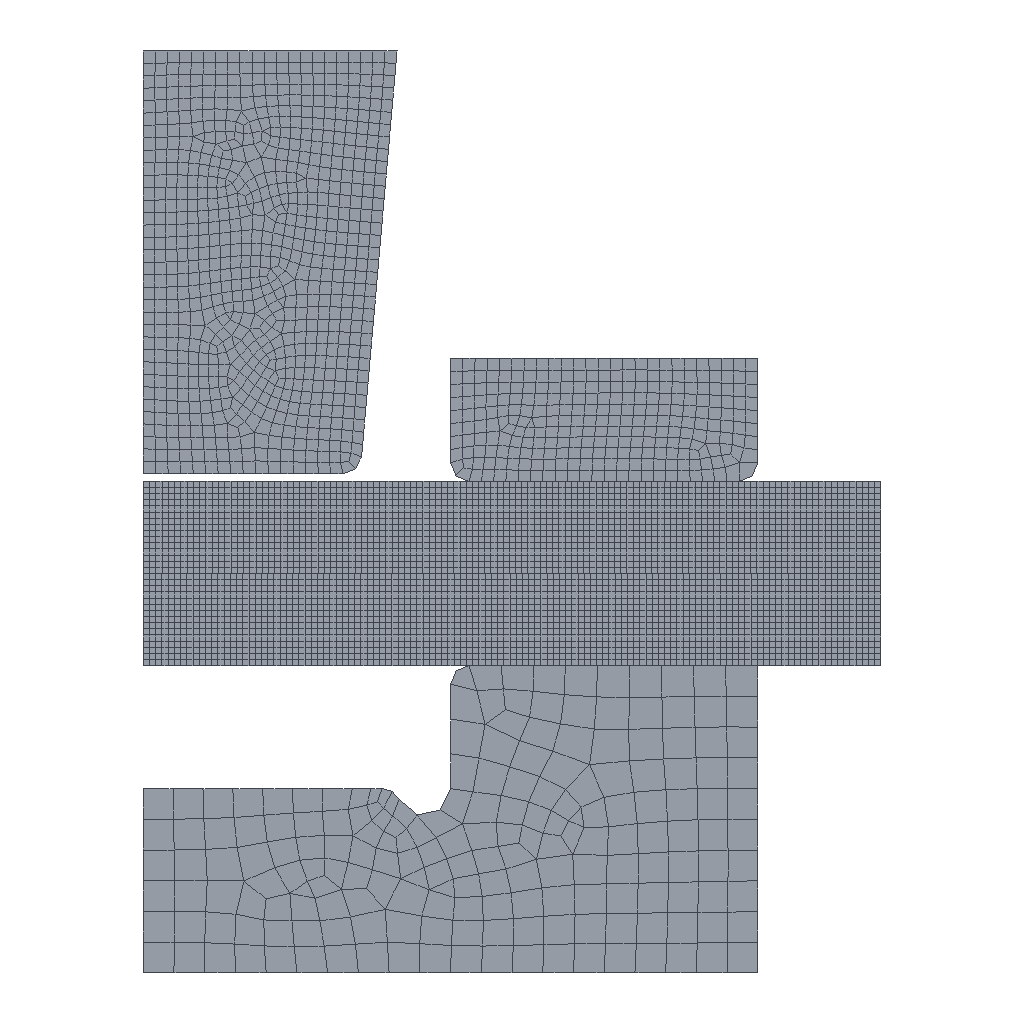Simulation study | abaqus
Set-up summary:
category,name,step,type,value,unit,region
solver,abaqus
solver,version,,,Abaqus/Explicit 2020
units,not stated in the deck,,not stated
analysis,deck,,dynamic temperature-displacement,dynamic temperature-displacement
load_step,Step-1,Step-1,dynamic temperature-displacement
load_step,Step-2,Step-2,dynamic temperature-displacement
load_step,Step-3,Step-3,dynamic temperature-displacement
load_step,Step-4,Step-4,dynamic temperature-displacement
load_step,requested,,,4
mesh,nodes,,,5179
mesh,elements,,,4792
element_type,CAX3,,axisymmetric,15
element_type,CAX4R,,axisymmetric,1207
element_type,CAX4RT,,axisymmetric,3570
load,load commands in deck,,count,4
bc,support commands in deck,,count,21
material,MATERIAL-AL,,in results
material,MATERIAL-GANG,,in results
material,REGANG,,in results
material,YATOU,,in results
check,setup vs results,,match,"per instance, exact: element labels, types and connectivity; labels of the nodes the elements use; coordinates not compared"
Abaqus input file, long lists of numbers shortened:
*Heading
** Job name: Job-3 Model name: Model-1
** Generated by: Abaqus/CAE 2020
*Preprint, echo=NO, model=NO, history=NO, contact=NO
**
** PARTS
**
*Part, name=Part-6
*Node
      1,           0.,   3.001
      2,           0.,           0.
** (219 more lines like these left out)
*Element, type=CAX3
1, 157, 153, 156
2, 220, 182, 168
** (2 more lines like these left out)
*Element, type=CAX4R
  5,  15, 171,  73,  14
  6,  83,  19,  20,  85
** (184 more lines like these left out)
*Node
    222,    7.65,           5.,           0.
*Nset, nset=Part-6-RefPt_, internal
222,
*Nset, nset=Set-2, generate
   1,  221,    1
*Elset, elset=Set-2, generate
   1,  190,    1
*Nset, nset=Set-3, generate
   1,  221,    1
*Elset, elset=Set-3, generate
   1,  190,    1
*Nset, nset=Set-4, generate
   1,  221,    1
*Elset, elset=Set-4, generate
   1,  190,    1
** Section: yatou
*Solid Section, elset=Set-4, material=yatou
,
*End Part
**
*Part, name=Part-7
*Node
      1,           0.,   15.002
      2,   4.13,   15.002
** (812 more lines like these left out)
*Element, type=CAX3
 1, 575, 804, 574
 2, 489, 560, 556
** (8 more lines like these left out)
*Element, type=CAX4R
 11, 194, 274, 204, 192
 12, 110,  11,  10, 109
** (753 more lines like these left out)
*Node
    815,   2.065,   15.002,           0.
*Nset, nset=Part-7-RefPt_, internal
815,
*Nset, nset=Set-2, generate
   1,  814,    1
*Elset, elset=Set-2, generate
   1,  765,    1
*Nset, nset=Set-3, generate
   1,  814,    1
*Elset, elset=Set-3, generate
   1,  765,    1
** Section: yatou
*Solid Section, elset=Set-3, material=yatou
,
*End Part
**
*Part, name=Part-8
*Node
      1,   5.088,   8.088
      2,   5.3,           8.
** (299 more lines like these left out)
*Element, type=CAX3
1, 276, 274, 268
*Element, type=CAX4R
  2,  68,   2,   9,  69
  3, 148, 296,  69,  70
** (264 more lines like these left out)
*Node
    302,          7.5,          10.,           0.
*Nset, nset=Part-8-RefPt_, internal
302,
*Nset, nset=Set-3, generate
   1,  301,    1
*Elset, elset=Set-3, generate
   1,  267,    1
*Nset, nset=Set-4, generate
   1,  301,    1
*Elset, elset=Set-4, generate
   1,  267,    1
** Section: yatou
*Solid Section, elset=Set-4, material=yatou
,
*End Part
**
*Part, name=Part-shang
*End Part
**
*Part, name=Part-xia
*End Part
**
**
** ASSEMBLY
**
*Assembly, name=Assembly
**
*Instance, name=Part-shang-1, part=Part-shang
*Node
      1,   6.36,           8.
      2,   6.36,          6.5
** (1918 more lines like these left out)
*Element, type=CAX4RT
  1,    1,    9,  297,  146
  2,    9,   10,  298,  297
** (1783 more lines like these left out)
*Nset, nset=Set-1, generate
    1,  1920,     1
*Elset, elset=Set-1, generate
    1,  1785,     1
*Nset, nset=_PickedSet36, internal, generate
    1,  1920,     1
*Elset, elset=_PickedSet36, internal, generate
    1,  1785,     1
** Section: Section-AL
*Solid Section, elset=_PickedSet36, material=Material-AL
,
*End Instance
**
*Instance, name=Part-xia-1, part=Part-xia
*Node
      1,   6.17,          6.5
      2,   6.17,           5.
** (1918 more lines like these left out)
*Element, type=CAX4RT
  1,    1,    9,  297,  150
  2,    9,   10,  298,  297
** (1783 more lines like these left out)
*Nset, nset=_PickedSet2, internal, generate
    1,  1920,     1
*Elset, elset=_PickedSet2, internal, generate
    1,  1785,     1
*Nset, nset=_PickedSet33, internal, generate
    1,  1920,     1
*Elset, elset=_PickedSet33, internal, generate
    1,  1785,     1
** Section: reg
*Solid Section, elset=_PickedSet33, material=regang
,
*End Instance
**
*Instance, name=Part-6-1, part=Part-6
*End Instance
**
*Instance, name=Part-7-1, part=Part-7
*End Instance
**
*Instance, name=Part-8-1, part=Part-8
*End Instance
**
*Nset, nset=Set-31, instance=Part-shang-1, generate
    1,  1920,     1
*Elset, elset=Set-31, instance=Part-shang-1, generate
    1,  1785,     1
*Nset, nset=Set-32, instance=Part-xia-1, generate
    1,  1920,     1
*Elset, elset=Set-32, instance=Part-xia-1, generate
    1,  1785,     1
*Nset, nset=Set-33, instance=Part-shang-1
  3,  4, 78, 79, 80, 81, 82, 83, 84, 85, 86, 87, 88, 89, 90, 91
*Nset, nset=Set-33, instance=Part-xia-1
  3,  4, 80, 81, 82, 83, 84, 85, 86, 87, 88, 89, 90, 91, 92, 93
*Elset, elset=Set-33, instance=Part-shang-1, generate
 826,  840,    1
*Elset, elset=Set-33, instance=Part-xia-1, generate
 856,  870,    1
*Nset, nset=Set-36, instance=Part-8-1
 302,
*Nset, nset=Set-37, instance=Part-6-1
 222,
*Nset, nset=Set-38, instance=Part-7-1
 815,
*Nset, nset=Set-39, instance=Part-7-1
 815,
*Nset, nset=Set-40, instance=Part-7-1
 815,
*Nset, nset=Set-41, instance=Part-8-1
 302,
*Nset, nset=b_Set-33, instance=Part-7-1, generate
   1,  814,    1
*Elset, elset=b_Set-33, instance=Part-7-1, generate
   1,  765,    1
*Nset, nset=b_Set-34, instance=Part-8-1, generate
   1,  301,    1
*Elset, elset=b_Set-34, instance=Part-8-1, generate
   1,  267,    1
*Nset, nset=b_Set-35, instance=Part-6-1, generate
   1,  221,    1
*Elset, elset=b_Set-35, instance=Part-6-1, generate
   1,  190,    1
*Nset, nset=congface, instance=Part-shang-1
    1,    4,    6,    7,    9,   10,   11,   12,   13,   14,   15,   16,   17,   18,   19,   20
   21,   22,   78,   79,   80,   81,   82,   83,   84,   85,   86,   87,   88,   89,   90,   91
** (111 more lines like these left out)
*Elset, elset=congface, instance=Part-shang-1, generate
    1,  1785,     1
*Elset, elset=down12345, instance=Part-xia-1
  893, 1186, 1200, 1486, 1500
*Nset, nset=downdown, instance=Part-xia-1
 1102, 1376, 1388, 1669, 1681
*Elset, elset=up12345, instance=Part-shang-1
 1097, 1110, 1163, 1456, 1470
*Nset, nset=upup, instance=Part-shang-1
 1291, 1304, 1368, 1641, 1654
*Nset, nset=zhuface, instance=Part-7-1, generate
   1,  815,    1
*Elset, elset=zhuface, instance=Part-7-1, generate
   1,  765,    1
*Nset, nset=_PickedSet129, internal, instance=Part-shang-1, generate
    1,  1920,     1
*Nset, nset=_PickedSet129, internal, instance=Part-xia-1, generate
    1,  1920,     1
*Elset, elset=_PickedSet129, internal, instance=Part-shang-1, generate
    1,  1785,     1
*Elset, elset=_PickedSet129, internal, instance=Part-xia-1, generate
    1,  1785,     1
*Nset, nset=_PickedSet130, internal, instance=Part-shang-1, generate
    1,  1920,     1
*Nset, nset=_PickedSet130, internal, instance=Part-xia-1, generate
    1,  1920,     1
*Elset, elset=_PickedSet130, internal, instance=Part-shang-1, generate
    1,  1785,     1
*Elset, elset=_PickedSet130, internal, instance=Part-xia-1, generate
    1,  1785,     1
*Nset, nset=_PickedSet131, internal, instance=Part-shang-1, generate
    1,  1920,     1
*Nset, nset=_PickedSet131, internal, instance=Part-xia-1, generate
    1,  1920,     1
*Elset, elset=_PickedSet131, internal, instance=Part-shang-1, generate
    1,  1785,     1
*Elset, elset=_PickedSet131, internal, instance=Part-xia-1, generate
    1,  1785,     1
*Nset, nset=_PickedSet132, internal, instance=Part-shang-1, generate
    1,  1920,     1
*Nset, nset=_PickedSet132, internal, instance=Part-xia-1, generate
    1,  1920,     1
*Elset, elset=_PickedSet132, internal, instance=Part-shang-1, generate
    1,  1785,     1
*Elset, elset=_PickedSet132, internal, instance=Part-xia-1, generate
    1,  1785,     1
*Nset, nset=_PickedSet148, internal, instance=Part-7-1
 815,
*Nset, nset=_PickedSet150, internal, instance=Part-8-1
 302,
*Nset, nset=_PickedSet152, internal, instance=Part-6-1
 222,
*Elset, elset=_Surf-34_S2, internal, instance=Part-shang-1, generate
   15,  1785,    15
*Elset, elset=_Surf-34_S2, internal, instance=Part-xia-1, generate
   15,  1785,    15
*Elset, elset=_Surf-34_S3, internal, instance=Part-shang-1
  826,  827,  828,  829,  830,  831,  832,  833,  834,  835,  836,  837,  838,  839,  840, 1126
 1127, 1128, 1129, 1130, 1131, 1132, 1133, 1134, 1135, 1136, 1137, 1138, 1139, 1140
*Elset, elset=_Surf-34_S3, internal, instance=Part-xia-1
  856,  857,  858,  859,  860,  861,  862,  863,  864,  865,  866,  867,  868,  869,  870, 1216
 1217, 1218, 1219, 1220, 1221, 1222, 1223, 1224, 1225, 1226, 1227, 1228, 1229, 1230
*Elset, elset=_Surf-34_S3, internal, instance=Part-6-1
 40, 44, 45, 46, 91
*Elset, elset=_Surf-34_S4, internal, instance=Part-shang-1, generate
    1,  1771,    15
*Elset, elset=_Surf-34_S4, internal, instance=Part-xia-1, generate
    1,  1771,    15
*Elset, elset=_Surf-34_S1, internal, instance=Part-6-1
  11,  43,  90, 136
*Surface, type=ELEMENT, name=Surf-34
_Surf-34_S2, S2
_Surf-34_S3, S3
_Surf-34_S4, S4
_Surf-34_S1, S1
*Elset, elset=_Surf-35_S2, internal, instance=Part-shang-1, generate
   15,  1785,    15
*Elset, elset=_Surf-35_S2, internal, instance=Part-xia-1, generate
   15,  1785,    15
*Elset, elset=_Surf-35_S3, internal, instance=Part-shang-1
  826,  827,  828,  829,  830,  831,  832,  833,  834,  835,  836,  837,  838,  839,  840, 1126
 1127, 1128, 1129, 1130, 1131, 1132, 1133, 1134, 1135, 1136, 1137, 1138, 1139, 1140
*Elset, elset=_Surf-35_S3, internal, instance=Part-xia-1
  856,  857,  858,  859,  860,  861,  862,  863,  864,  865,  866,  867,  868,  869,  870, 1216
 1217, 1218, 1219, 1220, 1221, 1222, 1223, 1224, 1225, 1226, 1227, 1228, 1229, 1230
*Elset, elset=_Surf-35_S4, internal, instance=Part-shang-1, generate
    1,  1771,    15
*Elset, elset=_Surf-35_S4, internal, instance=Part-xia-1, generate
    1,  1771,    15
*Surface, type=ELEMENT, name=Surf-35
_Surf-35_S2, S2
_Surf-35_S3, S3
_Surf-35_S4, S4
*Elset, elset=_Surf-36_S2, internal, instance=Part-shang-1, generate
   15,  1785,    15
*Elset, elset=_Surf-36_S2, internal, instance=Part-xia-1, generate
  885,  1230,    15
*Elset, elset=_Surf-36_S3, internal, instance=Part-shang-1
  826,  827,  828,  829,  830,  831,  832,  833,  834,  835,  836,  837,  838,  839,  840, 1126
 1127, 1128, 1129, 1130, 1131, 1132, 1133, 1134, 1135, 1136, 1137, 1138, 1139, 1140
*Elset, elset=_Surf-36_S3, internal, instance=Part-xia-1
  856,  857,  858,  859,  860,  861,  862,  863,  864,  865,  866,  867,  868,  869,  870, 1216
 1217, 1218, 1219, 1220, 1221, 1222, 1223, 1224, 1225, 1226, 1227, 1228, 1229, 1230
*Elset, elset=_Surf-36_S4, internal, instance=Part-shang-1, generate
    1,  1771,    15
*Elset, elset=_Surf-36_S4, internal, instance=Part-xia-1, generate
    1,  1771,    15
*Surface, type=ELEMENT, name=Surf-36
_Surf-36_S2, S2
_Surf-36_S3, S3
_Surf-36_S4, S4
*Elset, elset=_cong-faceaaa_S2, internal, instance=Part-shang-1, generate
  855,  1140,    15
*Elset, elset=_cong-faceaaa_S4, internal, instance=Part-shang-1, generate
 1141,  1771,    15
*Surface, type=ELEMENT, name=cong-faceaaa
_cong-faceaaa_S2, S2
_cong-faceaaa_S4, S4
*Elset, elset=_m_Surf-22_S2, internal, instance=Part-shang-1
   15,   30,   45,   60,   75,   90,  105,  120,  135,  150,  165,  180,  195,  210,  225,  240
  255,  270,  285,  300,  315,  330,  345,  360,  375,  390,  405,  420,  435,  450,  465,  480
** (5 more lines like these left out)
*Elset, elset=_m_Surf-22_S4, internal, instance=Part-shang-1, generate
  841,  1126,    15
*Surface, type=ELEMENT, name=m_Surf-22
_m_Surf-22_S2, S2
_m_Surf-22_S4, S4
*Elset, elset=_m_Surf-30_S2, internal, instance=Part-shang-1
   15,   30,   45,   60,   75,   90,  105,  120,  135,  150,  165,  180,  195,  210,  225,  240
  255,  270,  285,  300,  315,  330,  345,  360,  375,  390,  405,  420,  435,  450,  465,  480
** (5 more lines like these left out)
*Elset, elset=_m_Surf-30_S4, internal, instance=Part-shang-1, generate
  841,  1126,    15
*Surface, type=ELEMENT, name=m_Surf-30
_m_Surf-30_S2, S2
_m_Surf-30_S4, S4
*Elset, elset=_s_Surf-22_S4, internal, instance=Part-xia-1
    1,   16,   31,   46,   61,   76,   91,  106,  121,  136,  151,  166,  181,  196,  211,  226
  241,  256,  271,  286,  301,  316,  331,  346,  361,  376,  391,  406,  421,  436,  451,  466
** (4 more lines like these left out)
*Elset, elset=_s_Surf-22_S2, internal, instance=Part-xia-1, generate
  885,  1230,    15
*Surface, type=ELEMENT, name=s_Surf-22
_s_Surf-22_S4, S4
_s_Surf-22_S2, S2
*Elset, elset=_s_Surf-24_S4, internal, instance=Part-shang-1
    1,   16,   31,   46,   61,   76,   91,  106,  121,  136,  151,  166,  181,  196,  211,  226
  241,  256,  271,  286,  301,  316,  331,  346,  361,  376,  391,  406,  421,  436,  451,  466
** (5 more lines like these left out)
*Surface, type=ELEMENT, name=s_Surf-24
_s_Surf-24_S4, S4
*Elset, elset=_s_Surf-26_S2, internal, instance=Part-xia-1
   15,   30,   45,   60,   75,   90,  105,  120,  135,  150,  165,  180,  195,  210,  225,  240
  255,  270,  285,  300,  315,  330,  345,  360,  375,  390,  405,  420,  435,  450,  465,  480
** (4 more lines like these left out)
*Surface, type=ELEMENT, name=s_Surf-26
_s_Surf-26_S2, S2
*Elset, elset=_s_Surf-28_S2, internal, instance=Part-shang-1, generate
  855,  1140,    15
*Surface, type=ELEMENT, name=s_Surf-28
_s_Surf-28_S2, S2
*Elset, elset=_s_Surf-30_S4, internal, instance=Part-xia-1
    1,   16,   31,   46,   61,   76,   91,  106,  121,  136,  151,  166,  181,  196,  211,  226
  241,  256,  271,  286,  301,  316,  331,  346,  361,  376,  391,  406,  421,  436,  451,  466
** (4 more lines like these left out)
*Elset, elset=_s_Surf-30_S2, internal, instance=Part-xia-1, generate
  885,  1230,    15
*Surface, type=ELEMENT, name=s_Surf-30
_s_Surf-30_S4, S4
_s_Surf-30_S2, S2
*Elset, elset=_zhu-faceaa_S1, internal, instance=Part-7-1
  15,  16,  17,  18,  22,  28,  36,  48,  58,  59,  78, 105, 117, 118, 121, 141
 146, 150, 159
*Elset, elset=_zhu-faceaa_S3, internal, instance=Part-7-1
  38,  41,  46,  50,  55,  57,  60,  62,  63, 102, 103, 104, 119, 154, 230
*Elset, elset=_zhu-faceaa_S2, internal, instance=Part-7-1
  27,  54,  56,  61,  65,  72,  73,  84,  88,  90,  92,  93,  94,  96,  97,  98
 100, 113, 114, 115, 122, 123, 126, 169, 171, 172, 182, 228
*Elset, elset=_zhu-faceaa_S4, internal, instance=Part-7-1
  14,  42,  45,  47,  49,  52,  63,  64,  68,  69,  70,  77,  79,  80,  89,  91
  95, 106, 107, 109, 124, 160, 179
*Surface, type=ELEMENT, name=zhu-faceaa
_zhu-faceaa_S1, S1
_zhu-faceaa_S3, S3
_zhu-faceaa_S2, S2
_zhu-faceaa_S4, S4
** Constraint: Constraint-1
*Rigid Body, ref node=_PickedSet148, elset=b_Set-33, position=CENTER OF MASS
** Constraint: Constraint-2
*Rigid Body, ref node=_PickedSet150, elset=b_Set-34, position=CENTER OF MASS
** Constraint: Constraint-3
*Rigid Body, ref node=_PickedSet152, elset=b_Set-35, position=CENTER OF MASS
*End Assembly
*Amplitude, name=Amp-1, definition=SMOOTH STEP
             0.,              0.,             0.8,              1.
*Amplitude, name=Amp-2, definition=SMOOTH STEP
             0.,              0.,          0.0135,              1.
*Amplitude, name=Amp-3
             0.,              0.,            0.01,              1.
**
** MATERIALS
**
*Material, name=Material-AL
*Conductivity
188.,
*Density
 2.796e-09,
*Elastic
70000., 0.341
*Expansion
 2.3e-05,
*Plastic, hardening=JOHNSON COOK
324., 114., 0.42, 1.34, 570.,  25.
*Rate Dependent, type=JOHNSON COOK
 0.002,1.
*Specific Heat
 9.6e+08,
*Material, name=Material-GANG
*Conductivity
30.,
*Density
 7.9e-09,
*Elastic
207000., 0.3
*Expansion
 1.3e-05,
*Plastic, hardening=JOHNSON COOK
500.,  600., 0.234,    1., 1500.,   25.
*Rate Dependent, type=JOHNSON COOK
 0.0134,1.
*Specific Heat
 5.9e+08,
*Material, name=regang
*Conductivity
 47.5,   0.
 47.5, 100.
 44.3, 200.
 41.8, 300.
 38.4, 400.
 37.1, 500.
 34.1, 600.
 30.6, 700.
 25.3, 800.
 26.7, 900.
 27.2,1000.
*Density
 7.9e-09,
*Elastic
210000., 0.283,    0.
206000., 0.287,  100.
200000.,  0.29,  200.
192000., 0.295,  300.
162000.,   0.3,  400.
155000., 0.303,  500.
150000.,  0.31,  600.
140000., 0.318,  700.
135000., 0.325,  800.
130000., 0.335,  900.
120000., 0.346, 1000.
*Expansion
 1.3e-05,
*Plastic
  162.,  0.,550.
  268., 0.1,550.
  309., 0.2,550.
  327., 0.3,550.
  335., 0.4,550.
  338., 0.5,550.
  142.,  0.,650.
  198., 0.1,650.
  234., 0.2,650.
  249., 0.3,650.
  256., 0.4,650.
 256.5, 0.5,650.
 120.2,  0.,750.
  168., 0.1,750.
  202., 0.2,750.
  217., 0.3,750.
  225., 0.4,750.
 225.5, 0.5,750.
  109.,  0.,800.
  141., 0.1,800.
  150., 0.2,800.
  163., 0.3,800.
  179., 0.4,800.
 179.6, 0.5,800.
  99.5,  0.,850.
  135., 0.1,850.
  152., 0.2,850.
  163., 0.3,850.
  168., 0.4,850.
  169., 0.5,850.
   89.,  0.,900.
  124., 0.1,900.
  141., 0.2,900.
  154., 0.3,900.
  159., 0.4,900.
  160., 0.5,900.
   80.,  0.,950.
  114., 0.1,950.
  121., 0.2,950.
  144., 0.3,950.
** (2 more lines like these left out)
*Specific Heat
 3.65e+08,   0.
 4.78e+08, 100.
 5.12e+08, 200.
  5.4e+08, 300.
  5.8e+08, 400.
 6.52e+08, 500.
  7.4e+08, 600.
  7.8e+08, 700.
 8.32e+08, 800.
 8.21e+08, 900.
 8.08e+08,1000.
*Material, name=yatou
*Conductivity
15.,
*Density
 9e-09,
*Elastic
600000., 0.2
*Specific Heat
 5.9e+08,
**
** INTERACTION PROPERTIES
**
*Film Property, name=AHTC
2.
*Surface Interaction, name=IHTC
*Friction
 0.35,
*Surface Behavior, pressure-overclosure=HARD
*Gap Conductance
10.,0.
 0.,1.
*Surface Interaction, name=IntProp-3
*Friction
 0.1,
*Surface Behavior, pressure-overclosure=HARD
*Film Property, name=chtc
200.
**
** PHYSICAL CONSTANTS
**
*Physical Constants, absolute zero=-273.15, stefan boltzmann=1.134e-09
**
** BOUNDARY CONDITIONS
**
** Name: die Type: Symmetric/Anti-symmetric/Fully fixed
*Boundary
Set-37, ENCASTRE
** Name: [REDACTED]
*Boundary
Set-40, 1, 1
Set-40, 2, 2
Set-40, 6, 6
** Name: [REDACTED]
*Boundary
Set-41, 1, 1
Set-41, 6, 6
**
** PREDEFINED FIELDS
**
** Name: Predefined Field-1   Type: Temperature
*Initial Conditions, type=TEMPERATURE
Set-31, 25.
** Name: Predefined Field-2   Type: Temperature
*Initial Conditions, type=TEMPERATURE
Set-32, 700.
**
** INTERACTIONS
**
** Interaction: Int-13
*Contact, op=NEW
*Contact Inclusions, ALL EXTERIOR
*Contact Property Assignment
 ,  , IntProp-3
** ----------------------------------------------------------------
**
** STEP: Step-1
**
*Step, name=Step-1, nlgeom=YES
*Dynamic Temperature-displacement, Explicit
, 0.0135
*Bulk Viscosity
0.06, 1.2
** Mass Scaling: Semi-Automatic
**               Whole Model
*Fixed Mass Scaling, factor=100.
**
** BOUNDARY CONDITIONS
**
** Name: die Type: Symmetric/Anti-symmetric/Fully fixed
*Boundary, op=NEW
Set-37, ENCASTRE
** Name: [REDACTED]
*Boundary, op=NEW
Set-40, 1, 1
Set-40, 2, 2
Set-40, 6, 6
** Name: [REDACTED]
*Boundary, op=NEW
Set-41, 1, 1
Set-41, 6, 6
*Adaptive Mesh Controls, name=Ada-1
1., 0., 0.
**
** LOADS
**
** Name: Load-2   Type: Concentrated force
*Cload, amplitude=Amp-3
Set-36, 2, -20000.
**
** INTERACTIONS
**
** Interaction: Int-5
*Contact Pair, interaction=IHTC, mechanical constraint=KINEMATIC, cpset=Int-5
m_Surf-30, s_Surf-30
**
** OUTPUT REQUESTS
**
*Restart, write, number interval=1, time marks=NO
**
** FIELD OUTPUT: F-Output-1
**
*Output, field
*Node Output
NT, RF, U, V
*Element Output, directions=YES
E, HFL, LE, MISES, PE, PEEQ, PEEQT, PEEQVAVG, S, STATUS, TEMP
*Contact Output
CDISP,
*Output, history, frequency=0
*End Step
** ----------------------------------------------------------------
**
** STEP: Step-2
**
*Step, name=Step-2, nlgeom=YES
*Dynamic Temperature-displacement, Explicit
, 0.59
*Bulk Viscosity
0.06, 1.2
** Mass Scaling: Semi-Automatic
**               Whole Model
*Fixed Mass Scaling, factor=100.
**
** BOUNDARY CONDITIONS
**
** Name: die Type: Symmetric/Anti-symmetric/Fully fixed
*Boundary, op=NEW
Set-37, ENCASTRE
** Name: [REDACTED]
*Boundary, op=NEW, amplitude=Amp-1
Set-40, 1, 1
Set-40, 2, 2, -4.5
Set-40, 6, 6
** Name: [REDACTED]
*Boundary, op=NEW
Set-41, 1, 1
Set-41, 6, 6
**
** OUTPUT REQUESTS
**
*Restart, write, number interval=1, time marks=NO
**
** FIELD OUTPUT: F-Output-1
**
*Output, field
*Node Output
NT, RF, U, V
*Element Output, directions=YES
E, HFL, LE, MISES, PE, PEEQ, PEEQT, PEEQVAVG, S, STATUS, TEMP
*Contact Output
CDISP,
**
** FIELD OUTPUT: F-Output-2
**
*Output, field, number interval=100
*Node Output
NT, RF, U, V
*Element Output, directions=YES
E, HFL, LE, MISES, PE, PEEQ, PEEQT, PEEQVAVG, S, STATUS, TEMP
*Contact Output
CDISP,
**
** HISTORY OUTPUT: H-Output-1
**
*Output, history, time interval=0.000295
*Node Output, nset=Set-40
RF1, RF2, U1, U2
*End Step
** ----------------------------------------------------------------
**
** STEP: Step-3
**
*Step, name=Step-3, nlgeom=YES
*Dynamic Temperature-displacement, Explicit
, 0.0135
*Bulk Viscosity
0.06, 1.2
**
** BOUNDARY CONDITIONS
**
** Name: [REDACTED]
*Boundary, amplitude=Amp-2
Set-40, 1, 1
Set-40, 2, 2, 3.9
Set-40, 6, 6
**
** INTERACTIONS
**
** Interaction: Int-13
*Contact, op=NEW
*Contact Inclusions, ALL EXTERIOR
*Contact Property Assignment
 ,  , IntProp-3
*Contact Formulation, type=PURE MASTER-SLAVE
zhu-faceaa , cong-faceaaa , MASTER
**
** OUTPUT REQUESTS
**
*Restart, write, number interval=1, time marks=NO
**
** FIELD OUTPUT: F-Output-1, F-Output-3
**
*Output, field
*Node Output
NT, RF, U, V
*Element Output, directions=YES
E, HFL, LE, MISES, PE, PEEQ, PEEQT, PEEQVAVG, S, STATUS, TEMP
*Contact Output
CDISP,
**
** FIELD OUTPUT: F-Output-2
**
*Output, field, number interval=100
*Node Output
NT, RF, U, V
*Element Output, directions=YES
E, HFL, LE, MISES, PE, PEEQ, PEEQT, PEEQVAVG, S, STATUS, TEMP
*Contact Output
CDISP,
**
** HISTORY OUTPUT: H-Output-down-all
**
*Output, history, time interval=6.75e-06
*Node Output, nset=downdown
NT,
**
** HISTORY OUTPUT: H-Output-all
**
*Node Output, nset=upup
NT,
*End Step
** ----------------------------------------------------------------
**
** STEP: Step-4
**
*Step, name=Step-4, nlgeom=YES
*Dynamic Temperature-displacement, Explicit
, 100.
*Bulk Viscosity
0.06, 1.2
** Mass Scaling: Semi-Automatic
**               Whole Model
*Fixed Mass Scaling, factor=500.
**
** INTERACTIONS
**
** Interaction: Int-6
*Sradiate
Surf-36, R, 25., 1.
**
** OUTPUT REQUESTS
**
*Restart, write, number interval=1, time marks=NO
**
** FIELD OUTPUT: F-Output-1, F-Output-3
**
*Output, field
*Node Output
NT, RF, U, V
*Element Output, directions=YES
E, HFL, LE, MISES, PE, PEEQ, PEEQT, PEEQVAVG, S, STATUS, TEMP
*Contact Output
CDISP,
**
** FIELD OUTPUT: F-Output-2
**
*Output, field, number interval=100
*Node Output
NT, RF, U, V
*Element Output, directions=YES
E, HFL, LE, MISES, PE, PEEQ, PEEQT, PEEQVAVG, S, STATUS, TEMP
*Contact Output
CDISP,
**
** HISTORY OUTPUT: H-Output-down-all
**
*Output, history, time interval=0.05
*Node Output, nset=downdown
NT,
**
** HISTORY OUTPUT: H-Output-all
**
*Node Output, nset=upup
NT,
*End Step
Results summary:
result,step,Step-1,completed,increments=100644 time=0.0135/0.0135
result,step,Step-2,completed,increments=15084865 time=0.59/0.59
result,step,Step-3,completed,increments=805048 time=0.0135/0.0135
result,step,Step-4,partial,increments=8461760 time=0.2841/100.0
result,analysis,,,"dynamic temperature-displacement, explict"
result,last_loadstep,,,4
result,primary field,,,"U, NT11"
result,reaction total,,FX,-2287.216,model units
result,reaction total,,FY,20004.383,model units
result,reaction total,,FZ,0.0,model units